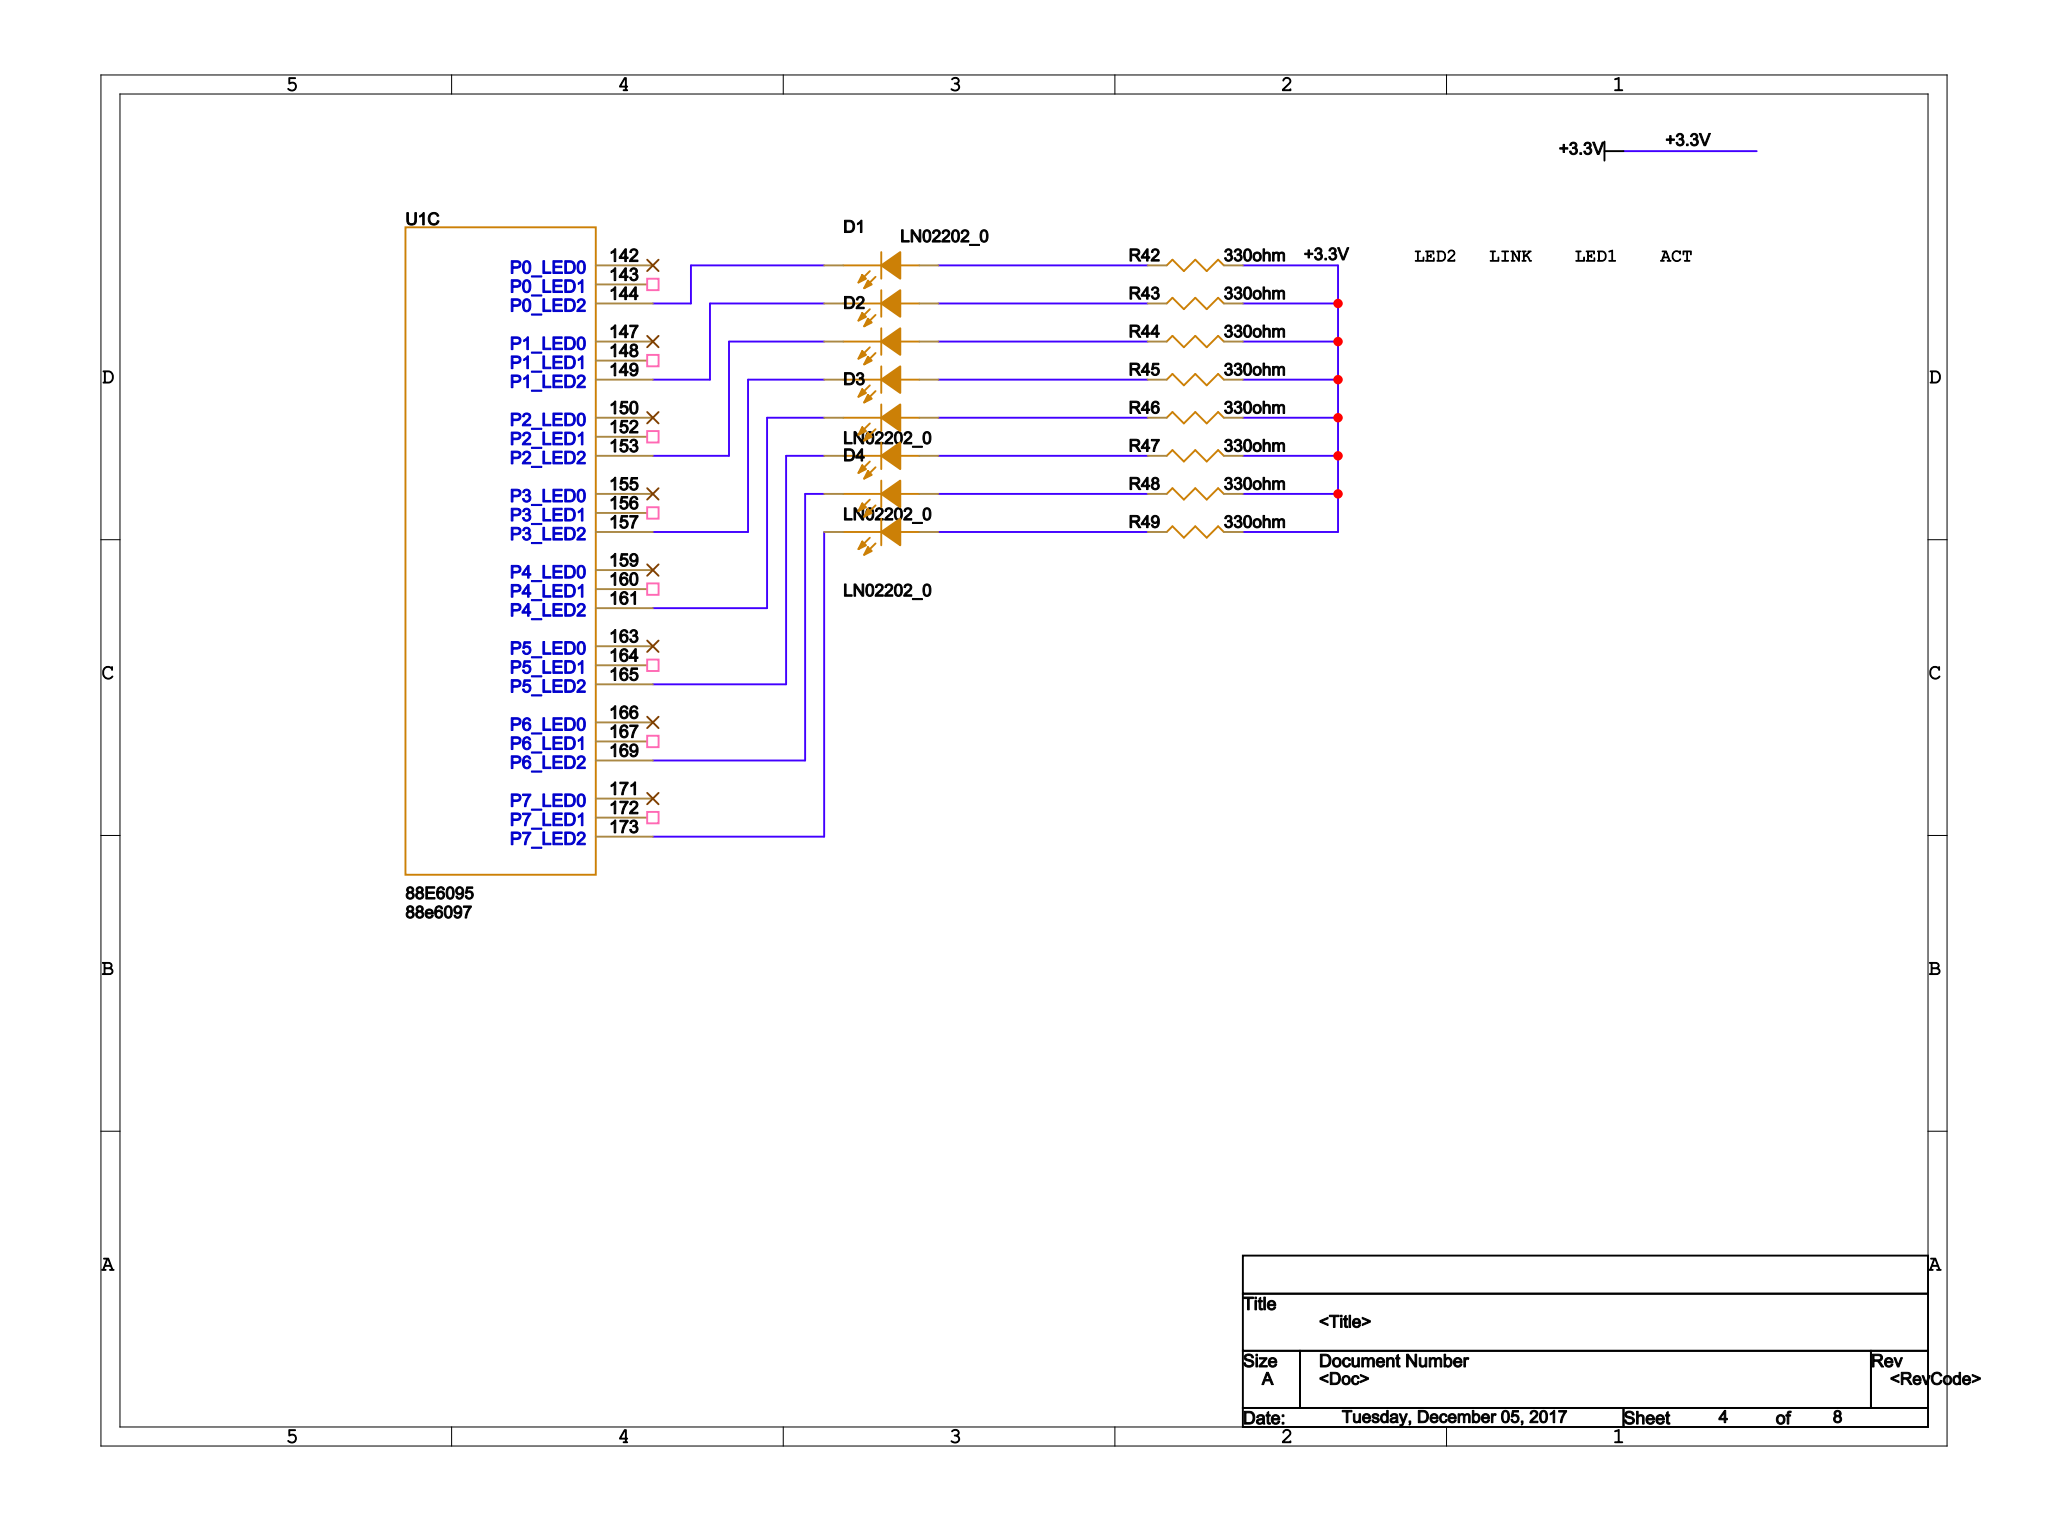Circuit board | Cadence Allegro | 219 parts | 174 nets | one sheet of the schematic
Parts on this sheet (reference | value | footprint):
D1 | LN02202_0 | LED_2
D2 | LN02202_0 | LED_2
D3 | LN02202_0 | LED_2
D4 | LN02202_0 | LED_2
R42 | 330ohm | SR0603
R43 | 330ohm | SR0603
R44 | 330ohm | SR0603
R45 | 330ohm | SR0603
R46 | 330ohm | SR0603
R47 | 330ohm | SR0603
R48 | 330ohm | SR0603
R49 | 330ohm | SR0603
U1 | 88E6095 | 88E6097
Nets of these parts (net: part-pin ...):
N1344528: D1-4 U1-144
N1345022: D1-2 U1-149
N1345038: D2-4 U1-153
N1345054: D2-2 U1-157
N1345073: D3-4 U1-161
N1345089: D3-2 U1-165
N1345108: D4-4 U1-169
N1345123: D4-2 U1-173
+3.3V: R42-2 R43-2 R44-2 R45-2 R46-2 R47-2 R48-2 R49-2
N1344518: D1-1 R43-1
N1344514: D1-3 R42-1
N1344596: D2-1 R45-1
N1344576: D2-3 R44-1
N1344660: D3-1 R47-1
N1344640: D3-3 R46-1
N1344724: D4-1 R49-1
N1344704: D4-3 R48-1